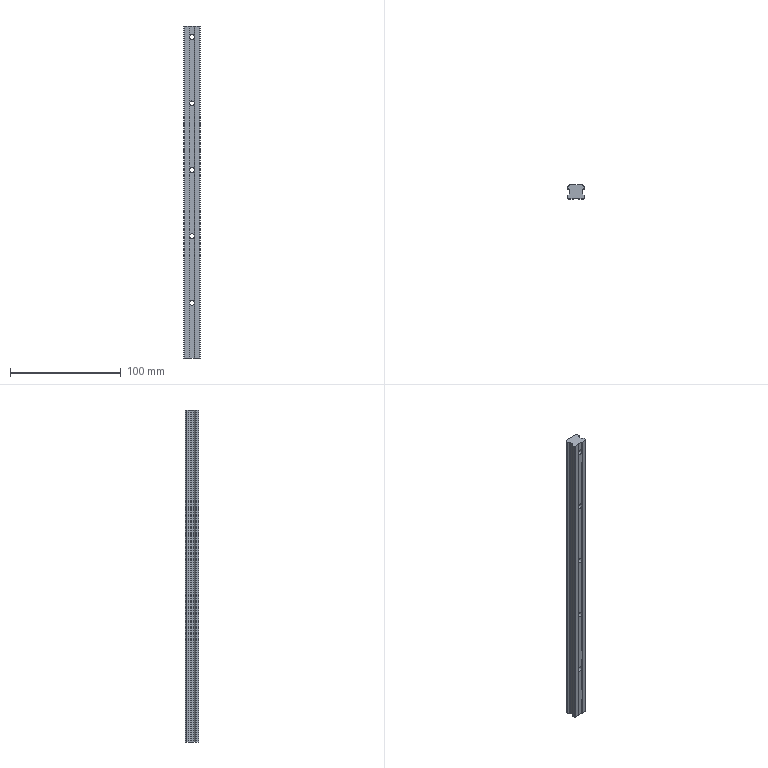Part | NX | 1 solid | 56 faces | box 15 x 12.5 x 300 mm | volume 47224 mm3 | plane 30 | cylinder 26 | commonest cylinder face diameters 0.6 x10 4.5 x5 8 x5 3 x4 1 x2